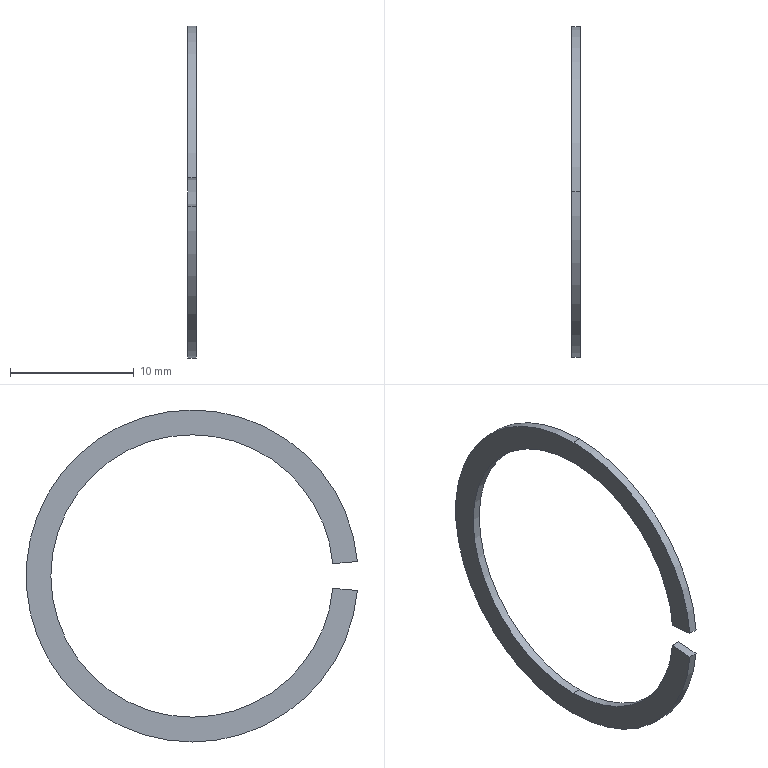Part | STEP file | 0243_Z_B6901ZZNR_2 | 1 solid | 10 faces | box 0.7 x 26.749 x 26.8 mm | volume 106.046 mm3 | cylinder 6 | plane 4 | commonest cylinder face diameters 22.8 x3 26.8 x3
STEP:
#1=CARTESIAN_POINT('',(0.,0.,0.));
#2=DIRECTION('',(0.,0.,1.));
#3=DIRECTION('',(1.,0.,0.));
#4=AXIS2_PLACEMENT_3D('',#1,#2,#3);
#5=CARTESIAN_POINT('',(1.75,0.,13.4));
#6=VERTEX_POINT('',#5);
#7=CARTESIAN_POINT('',(1.75,0.,-13.4));
#8=VERTEX_POINT('',#7);
#9=CARTESIAN_POINT('',(1.75,0.,0.));
#10=DIRECTION('',(-1.,0.,0.));
#11=DIRECTION('',(0.,0.,1.));
#12=AXIS2_PLACEMENT_3D('',#9,#10,#11);
#13=CIRCLE('',#12,13.4);
#14=CARTESIAN_POINT('',(1.05,0.,0.));
#15=DIRECTION('',(-1.,0.,0.));
#16=DIRECTION('',(0.,0.,1.));
#17=AXIS2_PLACEMENT_3D('',#14,#15,#16);
#18=CYLINDRICAL_SURFACE('',#17,13.4);
#19=CARTESIAN_POINT('',(0.,-0.7));
#20=DIRECTION('',(1.,0.));
#21=VECTOR('',#20,1.);
#22=LINE('',#19,#21);
#23=(GEOMETRIC_REPRESENTATION_CONTEXT(2)PARAMETRIC_REPRESENTATION_CONTEXT()REPRESENTATION_CONTEXT('',''));
#24=DEFINITIONAL_REPRESENTATION('',(#22),#23);
#25=PCURVE('',#18,#24);
#26=CARTESIAN_POINT('',(1.75,0.,0.));
#27=DIRECTION('',(1.,0.,0.));
#28=DIRECTION('',(0.,0.,-1.));
#29=AXIS2_PLACEMENT_3D('',#26,#27,#28);
#30=PLANE('',#29);
#31=CARTESIAN_POINT('',(-13.4,0.));
#32=CARTESIAN_POINT('',(-13.4,23.209));
#33=CARTESIAN_POINT('',(6.7,11.605));
#34=CARTESIAN_POINT('',(26.8,0.));
#35=CARTESIAN_POINT('',(6.7,-11.605));
#36=CARTESIAN_POINT('',(-13.4,-23.209));
#37=CARTESIAN_POINT('',(-13.4,0.));
#38=(BOUNDED_CURVE()B_SPLINE_CURVE(2,(#31,#32,#33,#34,#35,#36,#37),.UNSPECIFIED.,.T.,.F.)B_SPLINE_CURVE_WITH_KNOTS((1,2,2,2,2,1),(-2.094,0.,2.094,4.189,6.283,8.378),.UNSPECIFIED.)CURVE()GEOMETRIC_REPRESENTATION_ITEM()RATIONAL_B_SPLINE_CURVE((1.,0.5,1.,0.5,1.,0.5,1.))REPRESENTATION_ITEM(''));
#39=(GEOMETRIC_REPRESENTATION_CONTEXT(2)PARAMETRIC_REPRESENTATION_CONTEXT()REPRESENTATION_CONTEXT('',''));
#40=DEFINITIONAL_REPRESENTATION('',(#38),#39);
#41=PCURVE('',#30,#40);
#42=SURFACE_CURVE('',#13,(#25,#41),.PCURVE_S1.);
#43=EDGE_CURVE('',#6,#8,#42,.T.);
#44=ORIENTED_EDGE('',*,*,#43,.T.);
#45=CARTESIAN_POINT('',(1.05,0.,-13.4));
#46=VERTEX_POINT('',#45);
#47=CARTESIAN_POINT('',(1.05,0.,-13.4));
#48=DIRECTION('',(-1.,0.,0.));
#49=VECTOR('',#48,1.);
#50=LINE('',#47,#49);
#51=CARTESIAN_POINT('',(3.142,0.));
#52=DIRECTION('',(0.,1.));
#53=VECTOR('',#52,1.);
#54=LINE('',#51,#53);
#55=(GEOMETRIC_REPRESENTATION_CONTEXT(2)PARAMETRIC_REPRESENTATION_CONTEXT()REPRESENTATION_CONTEXT('',''));
#56=DEFINITIONAL_REPRESENTATION('',(#54),#55);
#57=PCURVE('',#18,#56);
#58=CARTESIAN_POINT('',(1.05,0.,0.));
#59=DIRECTION('',(-1.,0.,0.));
#60=DIRECTION('',(0.,0.,1.));
#61=AXIS2_PLACEMENT_3D('',#58,#59,#60);
#62=CYLINDRICAL_SURFACE('',#61,13.4);
#63=CARTESIAN_POINT('',(3.142,0.));
#64=DIRECTION('',(0.,1.));
#65=VECTOR('',#64,1.);
#66=LINE('',#63,#65);
#67=(GEOMETRIC_REPRESENTATION_CONTEXT(2)PARAMETRIC_REPRESENTATION_CONTEXT()REPRESENTATION_CONTEXT('',''));
#68=DEFINITIONAL_REPRESENTATION('',(#66),#67);
#69=PCURVE('',#62,#68);
#70=SURFACE_CURVE('',#50,(#57,#69),.PCURVE_S1.);
#71=EDGE_CURVE('',#8,#46,#70,.T.);
#72=ORIENTED_EDGE('',*,*,#71,.T.);
#73=CARTESIAN_POINT('',(1.05,0.,13.4));
#74=VERTEX_POINT('',#73);
#75=CARTESIAN_POINT('',(1.05,0.,0.));
#76=DIRECTION('',(1.,0.,0.));
#77=DIRECTION('',(0.,0.,1.));
#78=AXIS2_PLACEMENT_3D('',#75,#76,#77);
#79=CIRCLE('',#78,13.4);
#80=CARTESIAN_POINT('',(6.283,0.));
#81=DIRECTION('',(-1.,0.));
#82=VECTOR('',#81,1.);
#83=LINE('',#80,#82);
#84=(GEOMETRIC_REPRESENTATION_CONTEXT(2)PARAMETRIC_REPRESENTATION_CONTEXT()REPRESENTATION_CONTEXT('',''));
#85=DEFINITIONAL_REPRESENTATION('',(#83),#84);
#86=PCURVE('',#18,#85);
#87=CARTESIAN_POINT('',(1.05,0.,0.));
#88=DIRECTION('',(1.,0.,0.));
#89=DIRECTION('',(0.,0.,-1.));
#90=AXIS2_PLACEMENT_3D('',#87,#88,#89);
#91=PLANE('',#90);
#92=CARTESIAN_POINT('',(0.,0.));
#93=DIRECTION('',(-1.,0.));
#94=AXIS2_PLACEMENT_2D('',#92,#93);
#95=CIRCLE('',#94,13.4);
#96=(GEOMETRIC_REPRESENTATION_CONTEXT(2)PARAMETRIC_REPRESENTATION_CONTEXT()REPRESENTATION_CONTEXT('',''));
#97=DEFINITIONAL_REPRESENTATION('',(#95),#96);
#98=PCURVE('',#91,#97);
#99=SURFACE_CURVE('',#79,(#86,#98),.PCURVE_S1.);
#100=EDGE_CURVE('',#46,#74,#99,.T.);
#101=ORIENTED_EDGE('',*,*,#100,.T.);
#102=CARTESIAN_POINT('',(1.05,0.,13.4));
#103=DIRECTION('',(-1.,0.,0.));
#104=VECTOR('',#103,1.);
#105=LINE('',#102,#104);
#106=CARTESIAN_POINT('',(0.,0.));
#107=DIRECTION('',(0.,1.));
#108=VECTOR('',#107,1.);
#109=LINE('',#106,#108);
#110=(GEOMETRIC_REPRESENTATION_CONTEXT(2)PARAMETRIC_REPRESENTATION_CONTEXT()REPRESENTATION_CONTEXT('',''));
#111=DEFINITIONAL_REPRESENTATION('',(#109),#110);
#112=PCURVE('',#18,#111);
#113=CARTESIAN_POINT('',(1.05,0.,0.));
#114=DIRECTION('',(-1.,0.,0.));
#115=DIRECTION('',(0.,0.,1.));
#116=AXIS2_PLACEMENT_3D('',#113,#114,#115);
#117=CYLINDRICAL_SURFACE('',#116,13.4);
#118=CARTESIAN_POINT('',(6.283,0.));
#119=DIRECTION('',(0.,1.));
#120=VECTOR('',#119,1.);
#121=LINE('',#118,#120);
#122=(GEOMETRIC_REPRESENTATION_CONTEXT(2)PARAMETRIC_REPRESENTATION_CONTEXT()REPRESENTATION_CONTEXT('',''));
#123=DEFINITIONAL_REPRESENTATION('',(#121),#122);
#124=PCURVE('',#117,#123);
#125=SURFACE_CURVE('',#105,(#112,#124),.PCURVE_S1.);
#126=EDGE_CURVE('',#6,#74,#125,.T.);
#127=ORIENTED_EDGE('',*,*,#126,.F.);
#128=EDGE_LOOP('',(#44,#72,#101,#127));
#129=FACE_BOUND('',#128,.T.);
#130=ADVANCED_FACE('',(#129),#18,.T.);
#131=CARTESIAN_POINT('',(1.75,-13.349,1.168));
#132=VERTEX_POINT('',#131);
#133=CARTESIAN_POINT('',(1.75,0.,0.));
#134=DIRECTION('',(-1.,0.,0.));
#135=DIRECTION('',(0.,0.,1.));
#136=AXIS2_PLACEMENT_3D('',#133,#134,#135);
#137=CIRCLE('',#136,13.4);
#138=CARTESIAN_POINT('',(0.,-0.7));
#139=DIRECTION('',(1.,0.));
#140=VECTOR('',#139,1.);
#141=LINE('',#138,#140);
#142=(GEOMETRIC_REPRESENTATION_CONTEXT(2)PARAMETRIC_REPRESENTATION_CONTEXT()REPRESENTATION_CONTEXT('',''));
#143=DEFINITIONAL_REPRESENTATION('',(#141),#142);
#144=PCURVE('',#117,#143);
#145=CARTESIAN_POINT('',(-13.4,0.));
#146=CARTESIAN_POINT('',(-13.4,23.209));
#147=CARTESIAN_POINT('',(6.7,11.605));
#148=CARTESIAN_POINT('',(26.8,0.));
#149=CARTESIAN_POINT('',(6.7,-11.605));
#150=CARTESIAN_POINT('',(-13.4,-23.209));
#151=CARTESIAN_POINT('',(-13.4,0.));
#152=(BOUNDED_CURVE()B_SPLINE_CURVE(2,(#145,#146,#147,#148,#149,#150,#151),.UNSPECIFIED.,.T.,.F.)B_SPLINE_CURVE_WITH_KNOTS((1,2,2,2,2,1),(-2.094,0.,2.094,4.189,6.283,8.378),.UNSPECIFIED.)CURVE()GEOMETRIC_REPRESENTATION_ITEM()RATIONAL_B_SPLINE_CURVE((1.,0.5,1.,0.5,1.,0.5,1.))REPRESENTATION_ITEM(''));
#153=(GEOMETRIC_REPRESENTATION_CONTEXT(2)PARAMETRIC_REPRESENTATION_CONTEXT()REPRESENTATION_CONTEXT('',''));
#154=DEFINITIONAL_REPRESENTATION('',(#152),#153);
#155=PCURVE('',#30,#154);
#156=SURFACE_CURVE('',#137,(#144,#155),.PCURVE_S1.);
#157=EDGE_CURVE('',#132,#6,#156,.T.);
#158=ORIENTED_EDGE('',*,*,#157,.T.);
#159=ORIENTED_EDGE('',*,*,#126,.T.);
#160=CARTESIAN_POINT('',(1.05,-13.349,1.168));
#161=VERTEX_POINT('',#160);
#162=CARTESIAN_POINT('',(1.05,0.,0.));
#163=DIRECTION('',(1.,0.,0.));
#164=DIRECTION('',(0.,0.,1.));
#165=AXIS2_PLACEMENT_3D('',#162,#163,#164);
#166=CIRCLE('',#165,13.4);
#167=CARTESIAN_POINT('',(6.283,0.));
#168=DIRECTION('',(-1.,0.));
#169=VECTOR('',#168,1.);
#170=LINE('',#167,#169);
#171=(GEOMETRIC_REPRESENTATION_CONTEXT(2)PARAMETRIC_REPRESENTATION_CONTEXT()REPRESENTATION_CONTEXT('',''));
#172=DEFINITIONAL_REPRESENTATION('',(#170),#171);
#173=PCURVE('',#117,#172);
#174=CARTESIAN_POINT('',(0.,0.));
#175=DIRECTION('',(-1.,0.));
#176=AXIS2_PLACEMENT_2D('',#174,#175);
#177=CIRCLE('',#176,13.4);
#178=(GEOMETRIC_REPRESENTATION_CONTEXT(2)PARAMETRIC_REPRESENTATION_CONTEXT()REPRESENTATION_CONTEXT('',''));
#179=DEFINITIONAL_REPRESENTATION('',(#177),#178);
#180=PCURVE('',#91,#179);
#181=SURFACE_CURVE('',#166,(#173,#180),.PCURVE_S1.);
#182=EDGE_CURVE('',#74,#161,#181,.T.);
#183=ORIENTED_EDGE('',*,*,#182,.T.);
#184=CARTESIAN_POINT('',(1.05,-13.349,1.168));
#185=DIRECTION('',(-1.,0.,0.));
#186=VECTOR('',#185,1.);
#187=LINE('',#184,#186);
#188=CARTESIAN_POINT('',(4.8,0.));
#189=DIRECTION('',(0.,1.));
#190=VECTOR('',#189,1.);
#191=LINE('',#188,#190);
#192=(GEOMETRIC_REPRESENTATION_CONTEXT(2)PARAMETRIC_REPRESENTATION_CONTEXT()REPRESENTATION_CONTEXT('',''));
#193=DEFINITIONAL_REPRESENTATION('',(#191),#192);
#194=PCURVE('',#117,#193);
#195=CARTESIAN_POINT('',(1.05,-11.357,0.9936));
#196=DIRECTION('',(0.,-0.08716,-0.9962));
#197=DIRECTION('',(0.,0.9962,-0.08716));
#198=AXIS2_PLACEMENT_3D('',#195,#196,#197);
#199=PLANE('',#198);
#200=CARTESIAN_POINT('',(-2.,0.));
#201=DIRECTION('',(0.,-1.));
#202=VECTOR('',#201,1.);
#203=LINE('',#200,#202);
#204=(GEOMETRIC_REPRESENTATION_CONTEXT(2)PARAMETRIC_REPRESENTATION_CONTEXT()REPRESENTATION_CONTEXT('',''));
#205=DEFINITIONAL_REPRESENTATION('',(#203),#204);
#206=PCURVE('',#199,#205);
#207=SURFACE_CURVE('',#187,(#194,#206),.PCURVE_S1.);
#208=EDGE_CURVE('',#132,#161,#207,.T.);
#209=ORIENTED_EDGE('',*,*,#208,.F.);
#210=EDGE_LOOP('',(#158,#159,#183,#209));
#211=FACE_BOUND('',#210,.T.);
#212=ADVANCED_FACE('',(#211),#117,.T.);
#213=CARTESIAN_POINT('',(1.75,-11.357,-0.9936));
#214=VERTEX_POINT('',#213);
#215=CARTESIAN_POINT('',(1.05,-11.357,-0.9936));
#216=VERTEX_POINT('',#215);
#217=CARTESIAN_POINT('',(1.05,-11.357,-0.9936));
#218=DIRECTION('',(-1.,0.,0.));
#219=VECTOR('',#218,1.);
#220=LINE('',#217,#219);
#221=CARTESIAN_POINT('',(1.05,0.,0.));
#222=DIRECTION('',(-1.,0.,0.));
#223=DIRECTION('',(0.,0.,1.));
#224=AXIS2_PLACEMENT_3D('',#221,#222,#223);
#225=CYLINDRICAL_SURFACE('',#224,11.4);
#226=CARTESIAN_POINT('',(4.625,0.));
#227=DIRECTION('',(0.,1.));
#228=VECTOR('',#227,1.);
#229=LINE('',#226,#228);
#230=(GEOMETRIC_REPRESENTATION_CONTEXT(2)PARAMETRIC_REPRESENTATION_CONTEXT()REPRESENTATION_CONTEXT('',''));
#231=DEFINITIONAL_REPRESENTATION('',(#229),#230);
#232=PCURVE('',#225,#231);
#233=CARTESIAN_POINT('',(1.05,-13.349,-1.168));
#234=DIRECTION('',(0.,-0.08716,0.9962));
#235=DIRECTION('',(0.,-0.9962,-0.08716));
#236=AXIS2_PLACEMENT_3D('',#233,#234,#235);
#237=PLANE('',#236);
#238=CARTESIAN_POINT('',(-2.,0.));
#239=DIRECTION('',(0.,-1.));
#240=VECTOR('',#239,1.);
#241=LINE('',#238,#240);
#242=(GEOMETRIC_REPRESENTATION_CONTEXT(2)PARAMETRIC_REPRESENTATION_CONTEXT()REPRESENTATION_CONTEXT('',''));
#243=DEFINITIONAL_REPRESENTATION('',(#241),#242);
#244=PCURVE('',#237,#243);
#245=SURFACE_CURVE('',#220,(#232,#244),.PCURVE_S1.);
#246=EDGE_CURVE('',#214,#216,#245,.T.);
#247=ORIENTED_EDGE('',*,*,#246,.T.);
#248=CARTESIAN_POINT('',(1.05,0.,-11.4));
#249=VERTEX_POINT('',#248);
#250=CARTESIAN_POINT('',(1.05,0.,0.));
#251=DIRECTION('',(-1.,0.,0.));
#252=DIRECTION('',(0.,0.,1.));
#253=AXIS2_PLACEMENT_3D('',#250,#251,#252);
#254=CIRCLE('',#253,11.4);
#255=CARTESIAN_POINT('',(0.,0.));
#256=DIRECTION('',(1.,0.));
#257=VECTOR('',#256,1.);
#258=LINE('',#255,#257);
#259=(GEOMETRIC_REPRESENTATION_CONTEXT(2)PARAMETRIC_REPRESENTATION_CONTEXT()REPRESENTATION_CONTEXT('',''));
#260=DEFINITIONAL_REPRESENTATION('',(#258),#259);
#261=PCURVE('',#225,#260);
#262=CARTESIAN_POINT('',(-11.4,0.));
#263=CARTESIAN_POINT('',(-11.4,19.745));
#264=CARTESIAN_POINT('',(5.7,9.873));
#265=CARTESIAN_POINT('',(22.8,0.));
#266=CARTESIAN_POINT('',(5.7,-9.873));
#267=CARTESIAN_POINT('',(-11.4,-19.745));
#268=CARTESIAN_POINT('',(-11.4,0.));
#269=(BOUNDED_CURVE()B_SPLINE_CURVE(2,(#262,#263,#264,#265,#266,#267,#268),.UNSPECIFIED.,.T.,.F.)B_SPLINE_CURVE_WITH_KNOTS((1,2,2,2,2,1),(-2.094,0.,2.094,4.189,6.283,8.378),.UNSPECIFIED.)CURVE()GEOMETRIC_REPRESENTATION_ITEM()RATIONAL_B_SPLINE_CURVE((1.,0.5,1.,0.5,1.,0.5,1.))REPRESENTATION_ITEM(''));
#270=(GEOMETRIC_REPRESENTATION_CONTEXT(2)PARAMETRIC_REPRESENTATION_CONTEXT()REPRESENTATION_CONTEXT('',''));
#271=DEFINITIONAL_REPRESENTATION('',(#269),#270);
#272=PCURVE('',#91,#271);
#273=SURFACE_CURVE('',#254,(#261,#272),.PCURVE_S1.);
#274=EDGE_CURVE('',#249,#216,#273,.T.);
#275=ORIENTED_EDGE('',*,*,#274,.F.);
#276=CARTESIAN_POINT('',(1.75,0.,-11.4));
#277=VERTEX_POINT('',#276);
#278=CARTESIAN_POINT('',(1.05,0.,-11.4));
#279=DIRECTION('',(-1.,0.,0.));
#280=VECTOR('',#279,1.);
#281=LINE('',#278,#280);
#282=CARTESIAN_POINT('',(3.142,0.));
#283=DIRECTION('',(0.,1.));
#284=VECTOR('',#283,1.);
#285=LINE('',#282,#284);
#286=(GEOMETRIC_REPRESENTATION_CONTEXT(2)PARAMETRIC_REPRESENTATION_CONTEXT()REPRESENTATION_CONTEXT('',''));
#287=DEFINITIONAL_REPRESENTATION('',(#285),#286);
#288=PCURVE('',#225,#287);
#289=CARTESIAN_POINT('',(1.05,0.,0.));
#290=DIRECTION('',(-1.,0.,0.));
#291=DIRECTION('',(0.,0.,1.));
#292=AXIS2_PLACEMENT_3D('',#289,#290,#291);
#293=CYLINDRICAL_SURFACE('',#292,11.4);
#294=CARTESIAN_POINT('',(3.142,0.));
#295=DIRECTION('',(0.,1.));
#296=VECTOR('',#295,1.);
#297=LINE('',#294,#296);
#298=(GEOMETRIC_REPRESENTATION_CONTEXT(2)PARAMETRIC_REPRESENTATION_CONTEXT()REPRESENTATION_CONTEXT('',''));
#299=DEFINITIONAL_REPRESENTATION('',(#297),#298);
#300=PCURVE('',#293,#299);
#301=SURFACE_CURVE('',#281,(#288,#300),.PCURVE_S1.);
#302=EDGE_CURVE('',#277,#249,#301,.T.);
#303=ORIENTED_EDGE('',*,*,#302,.F.);
#304=CARTESIAN_POINT('',(1.75,0.,0.));
#305=DIRECTION('',(-1.,0.,0.));
#306=DIRECTION('',(0.,0.,1.));
#307=AXIS2_PLACEMENT_3D('',#304,#305,#306);
#308=CIRCLE('',#307,11.4);
#309=CARTESIAN_POINT('',(0.,-0.7));
#310=DIRECTION('',(1.,0.));
#311=VECTOR('',#310,1.);
#312=LINE('',#309,#311);
#313=(GEOMETRIC_REPRESENTATION_CONTEXT(2)PARAMETRIC_REPRESENTATION_CONTEXT()REPRESENTATION_CONTEXT('',''));
#314=DEFINITIONAL_REPRESENTATION('',(#312),#313);
#315=PCURVE('',#225,#314);
#316=CARTESIAN_POINT('',(-11.4,0.));
#317=CARTESIAN_POINT('',(-11.4,19.745));
#318=CARTESIAN_POINT('',(5.7,9.873));
#319=CARTESIAN_POINT('',(22.8,0.));
#320=CARTESIAN_POINT('',(5.7,-9.873));
#321=CARTESIAN_POINT('',(-11.4,-19.745));
#322=CARTESIAN_POINT('',(-11.4,0.));
#323=(BOUNDED_CURVE()B_SPLINE_CURVE(2,(#316,#317,#318,#319,#320,#321,#322),.UNSPECIFIED.,.T.,.F.)B_SPLINE_CURVE_WITH_KNOTS((1,2,2,2,2,1),(-2.094,0.,2.094,4.189,6.283,8.378),.UNSPECIFIED.)CURVE()GEOMETRIC_REPRESENTATION_ITEM()RATIONAL_B_SPLINE_CURVE((1.,0.5,1.,0.5,1.,0.5,1.))REPRESENTATION_ITEM(''));
#324=(GEOMETRIC_REPRESENTATION_CONTEXT(2)PARAMETRIC_REPRESENTATION_CONTEXT()REPRESENTATION_CONTEXT('',''));
#325=DEFINITIONAL_REPRESENTATION('',(#323),#324);
#326=PCURVE('',#30,#325);
#327=SURFACE_CURVE('',#308,(#315,#326),.PCURVE_S1.);
#328=EDGE_CURVE('',#277,#214,#327,.T.);
#329=ORIENTED_EDGE('',*,*,#328,.T.);
#330=EDGE_LOOP('',(#247,#275,#303,#329));
#331=FACE_BOUND('',#330,.F.);
#332=ADVANCED_FACE('',(#331),#225,.F.);
#333=CARTESIAN_POINT('',(1.05,0.,11.4));
#334=VERTEX_POINT('',#333);
#335=CARTESIAN_POINT('',(1.05,0.,0.));
#336=DIRECTION('',(-1.,0.,0.));
#337=DIRECTION('',(0.,0.,1.));
#338=AXIS2_PLACEMENT_3D('',#335,#336,#337);
#339=CIRCLE('',#338,11.4);
#340=CARTESIAN_POINT('',(0.,0.));
#341=DIRECTION('',(1.,0.));
#342=VECTOR('',#341,1.);
#343=LINE('',#340,#342);
#344=(GEOMETRIC_REPRESENTATION_CONTEXT(2)PARAMETRIC_REPRESENTATION_CONTEXT()REPRESENTATION_CONTEXT('',''));
#345=DEFINITIONAL_REPRESENTATION('',(#343),#344);
#346=PCURVE('',#293,#345);
#347=CARTESIAN_POINT('',(-11.4,0.));
#348=CARTESIAN_POINT('',(-11.4,19.745));
#349=CARTESIAN_POINT('',(5.7,9.873));
#350=CARTESIAN_POINT('',(22.8,0.));
#351=CARTESIAN_POINT('',(5.7,-9.873));
#352=CARTESIAN_POINT('',(-11.4,-19.745));
#353=CARTESIAN_POINT('',(-11.4,0.));
#354=(BOUNDED_CURVE()B_SPLINE_CURVE(2,(#347,#348,#349,#350,#351,#352,#353),.UNSPECIFIED.,.T.,.F.)B_SPLINE_CURVE_WITH_KNOTS((1,2,2,2,2,1),(-2.094,0.,2.094,4.189,6.283,8.378),.UNSPECIFIED.)CURVE()GEOMETRIC_REPRESENTATION_ITEM()RATIONAL_B_SPLINE_CURVE((1.,0.5,1.,0.5,1.,0.5,1.))REPRESENTATION_ITEM(''));
#355=(GEOMETRIC_REPRESENTATION_CONTEXT(2)PARAMETRIC_REPRESENTATION_CONTEXT()REPRESENTATION_CONTEXT('',''));
#356=DEFINITIONAL_REPRESENTATION('',(#354),#355);
#357=PCURVE('',#91,#356);
#358=SURFACE_CURVE('',#339,(#346,#357),.PCURVE_S1.);
#359=EDGE_CURVE('',#334,#249,#358,.T.);
#360=ORIENTED_EDGE('',*,*,#359,.F.);
#361=CARTESIAN_POINT('',(1.75,0.,11.4));
#362=VERTEX_POINT('',#361);
#363=CARTESIAN_POINT('',(1.05,0.,11.4));
#364=DIRECTION('',(-1.,0.,0.));
#365=VECTOR('',#364,1.);
#366=LINE('',#363,#365);
#367=CARTESIAN_POINT('',(0.,0.));
#368=DIRECTION('',(0.,1.));
#369=VECTOR('',#368,1.);
#370=LINE('',#367,#369);
#371=(GEOMETRIC_REPRESENTATION_CONTEXT(2)PARAMETRIC_REPRESENTATION_CONTEXT()REPRESENTATION_CONTEXT('',''));
#372=DEFINITIONAL_REPRESENTATION('',(#370),#371);
#373=PCURVE('',#293,#372);
#374=CARTESIAN_POINT('',(1.05,0.,0.));
#375=DIRECTION('',(-1.,0.,0.));
#376=DIRECTION('',(0.,0.,1.));
#377=AXIS2_PLACEMENT_3D('',#374,#375,#376);
#378=CYLINDRICAL_SURFACE('',#377,11.4);
#379=CARTESIAN_POINT('',(6.283,0.));
#380=DIRECTION('',(0.,1.));
#381=VECTOR('',#380,1.);
#382=LINE('',#379,#381);
#383=(GEOMETRIC_REPRESENTATION_CONTEXT(2)PARAMETRIC_REPRESENTATION_CONTEXT()REPRESENTATION_CONTEXT('',''));
#384=DEFINITIONAL_REPRESENTATION('',(#382),#383);
#385=PCURVE('',#378,#384);
#386=SURFACE_CURVE('',#366,(#373,#385),.PCURVE_S1.);
#387=EDGE_CURVE('',#362,#334,#386,.T.);
#388=ORIENTED_EDGE('',*,*,#387,.F.);
#389=CARTESIAN_POINT('',(1.75,0.,0.));
#390=DIRECTION('',(-1.,0.,0.));
#391=DIRECTION('',(0.,0.,1.));
#392=AXIS2_PLACEMENT_3D('',#389,#390,#391);
#393=CIRCLE('',#392,11.4);
#394=CARTESIAN_POINT('',(0.,-0.7));
#395=DIRECTION('',(1.,0.));
#396=VECTOR('',#395,1.);
#397=LINE('',#394,#396);
#398=(GEOMETRIC_REPRESENTATION_CONTEXT(2)PARAMETRIC_REPRESENTATION_CONTEXT()REPRESENTATION_CONTEXT('',''));
#399=DEFINITIONAL_REPRESENTATION('',(#397),#398);
#400=PCURVE('',#293,#399);
#401=CARTESIAN_POINT('',(-11.4,0.));
#402=CARTESIAN_POINT('',(-11.4,19.745));
#403=CARTESIAN_POINT('',(5.7,9.873));
#404=CARTESIAN_POINT('',(22.8,0.));
#405=CARTESIAN_POINT('',(5.7,-9.873));
#406=CARTESIAN_POINT('',(-11.4,-19.745));
#407=CARTESIAN_POINT('',(-11.4,0.));
#408=(BOUNDED_CURVE()B_SPLINE_CURVE(2,(#401,#402,#403,#404,#405,#406,#407),.UNSPECIFIED.,.T.,.F.)B_SPLINE_CURVE_WITH_KNOTS((1,2,2,2,2,1),(-2.094,0.,2.094,4.189,6.283,8.378),.UNSPECIFIED.)CURVE()GEOMETRIC_REPRESENTATION_ITEM()RATIONAL_B_SPLINE_CURVE((1.,0.5,1.,0.5,1.,0.5,1.))REPRESENTATION_ITEM(''));
#409=(GEOMETRIC_REPRESENTATION_CONTEXT(2)PARAMETRIC_REPRESENTATION_CONTEXT()REPRESENTATION_CONTEXT('',''));
#410=DEFINITIONAL_REPRESENTATION('',(#408),#409);
#411=PCURVE('',#30,#410);
#412=SURFACE_CURVE('',#393,(#400,#411),.PCURVE_S1.);
#413=EDGE_CURVE('',#362,#277,#412,.T.);
#414=ORIENTED_EDGE('',*,*,#413,.T.);
#415=ORIENTED_EDGE('',*,*,#302,.T.);
#416=EDGE_LOOP('',(#360,#388,#414,#415));
#417=FACE_BOUND('',#416,.F.);
#418=ADVANCED_FACE('',(#417),#293,.F.);
#419=CARTESIAN_POINT('',(1.05,-13.349,-1.168));
#420=VERTEX_POINT('',#419);
#421=CARTESIAN_POINT('',(1.05,-11.357,-0.9936));
#422=DIRECTION('',(0.,-0.9962,-0.08716));
#423=VECTOR('',#422,1.);
#424=LINE('',#421,#423);
#425=CARTESIAN_POINT('',(0.9936,-11.357));
#426=DIRECTION('',(0.08716,-0.9962));
#427=VECTOR('',#426,1.);
#428=LINE('',#425,#427);
#429=(GEOMETRIC_REPRESENTATION_CONTEXT(2)PARAMETRIC_REPRESENTATION_CONTEXT()REPRESENTATION_CONTEXT('',''));
#430=DEFINITIONAL_REPRESENTATION('',(#428),#429);
#431=PCURVE('',#91,#430);
#432=CARTESIAN_POINT('',(-2.,0.));
#433=DIRECTION('',(1.,0.));
#434=VECTOR('',#433,1.);
#435=LINE('',#432,#434);
#436=(GEOMETRIC_REPRESENTATION_CONTEXT(2)PARAMETRIC_REPRESENTATION_CONTEXT()REPRESENTATION_CONTEXT('',''));
#437=DEFINITIONAL_REPRESENTATION('',(#435),#436);
#438=PCURVE('',#237,#437);
#439=SURFACE_CURVE('',#424,(#431,#438),.PCURVE_S1.);
#440=EDGE_CURVE('',#216,#420,#439,.T.);
#441=ORIENTED_EDGE('',*,*,#440,.F.);
#442=ORIENTED_EDGE('',*,*,#274,.F.);
#443=ORIENTED_EDGE('',*,*,#359,.F.);
#444=CARTESIAN_POINT('',(1.05,-11.357,0.9936));
#445=VERTEX_POINT('',#444);
#446=CARTESIAN_POINT('',(1.05,0.,0.));
#447=DIRECTION('',(-1.,0.,0.));
#448=DIRECTION('',(0.,0.,1.));
#449=AXIS2_PLACEMENT_3D('',#446,#447,#448);
#450=CIRCLE('',#449,11.4);
#451=CARTESIAN_POINT('',(-11.4,0.));
#452=CARTESIAN_POINT('',(-11.4,19.745));
#453=CARTESIAN_POINT('',(5.7,9.873));
#454=CARTESIAN_POINT('',(22.8,0.));
#455=CARTESIAN_POINT('',(5.7,-9.873));
#456=CARTESIAN_POINT('',(-11.4,-19.745));
#457=CARTESIAN_POINT('',(-11.4,0.));
#458=(BOUNDED_CURVE()B_SPLINE_CURVE(2,(#451,#452,#453,#454,#455,#456,#457),.UNSPECIFIED.,.T.,.F.)B_SPLINE_CURVE_WITH_KNOTS((1,2,2,2,2,1),(-2.094,0.,2.094,4.189,6.283,8.378),.UNSPECIFIED.)CURVE()GEOMETRIC_REPRESENTATION_ITEM()RATIONAL_B_SPLINE_CURVE((1.,0.5,1.,0.5,1.,0.5,1.))REPRESENTATION_ITEM(''));
#459=(GEOMETRIC_REPRESENTATION_CONTEXT(2)PARAMETRIC_REPRESENTATION_CONTEXT()REPRESENTATION_CONTEXT('',''));
#460=DEFINITIONAL_REPRESENTATION('',(#458),#459);
#461=PCURVE('',#91,#460);
#462=CARTESIAN_POINT('',(0.,0.));
#463=DIRECTION('',(1.,0.));
#464=VECTOR('',#463,1.);
#465=LINE('',#462,#464);
#466=(GEOMETRIC_REPRESENTATION_CONTEXT(2)PARAMETRIC_REPRESENTATION_CONTEXT()REPRESENTATION_CONTEXT('',''));
#467=DEFINITIONAL_REPRESENTATION('',(#465),#466);
#468=PCURVE('',#378,#467);
#469=SURFACE_CURVE('',#450,(#461,#468),.PCURVE_S1.);
#470=EDGE_CURVE('',#445,#334,#469,.T.);
#471=ORIENTED_EDGE('',*,*,#470,.F.);
#472=CARTESIAN_POINT('',(1.05,-13.349,1.168));
#473=DIRECTION('',(0.,0.9962,-0.08716));
#474=VECTOR('',#473,1.);
#475=LINE('',#472,#474);
#476=CARTESIAN_POINT('',(-1.168,-13.349));
#477=DIRECTION('',(0.08716,0.9962));
#478=VECTOR('',#477,1.);
#479=LINE('',#476,#478);
#480=(GEOMETRIC_REPRESENTATION_CONTEXT(2)PARAMETRIC_REPRESENTATION_CONTEXT()REPRESENTATION_CONTEXT('',''));
#481=DEFINITIONAL_REPRESENTATION('',(#479),#480);
#482=PCURVE('',#91,#481);
#483=CARTESIAN_POINT('',(-2.,0.));
#484=DIRECTION('',(1.,0.));
#485=VECTOR('',#484,1.);
#486=LINE('',#483,#485);
#487=(GEOMETRIC_REPRESENTATION_CONTEXT(2)PARAMETRIC_REPRESENTATION_CONTEXT()REPRESENTATION_CONTEXT('',''));
#488=DEFINITIONAL_REPRESENTATION('',(#486),#487);
#489=PCURVE('',#199,#488);
#490=SURFACE_CURVE('',#475,(#482,#489),.PCURVE_S1.);
#491=EDGE_CURVE('',#161,#445,#490,.T.);
#492=ORIENTED_EDGE('',*,*,#491,.F.);
#493=ORIENTED_EDGE('',*,*,#182,.F.);
#494=ORIENTED_EDGE('',*,*,#100,.F.);
#495=CARTESIAN_POINT('',(1.05,0.,0.));
#496=DIRECTION('',(1.,0.,0.));
#497=DIRECTION('',(0.,0.,1.));
#498=AXIS2_PLACEMENT_3D('',#495,#496,#497);
#499=CIRCLE('',#498,13.4);
#500=CARTESIAN_POINT('',(0.,0.));
#501=DIRECTION('',(-1.,0.));
#502=AXIS2_PLACEMENT_2D('',#500,#501);
#503=CIRCLE('',#502,13.4);
#504=(GEOMETRIC_REPRESENTATION_CONTEXT(2)PARAMETRIC_REPRESENTATION_CONTEXT()REPRESENTATION_CONTEXT('',''));
#505=DEFINITIONAL_REPRESENTATION('',(#503),#504);
#506=PCURVE('',#91,#505);
#507=CARTESIAN_POINT('',(6.283,0.));
#508=DIRECTION('',(-1.,0.));
#509=VECTOR('',#508,1.);
#510=LINE('',#507,#509);
#511=(GEOMETRIC_REPRESENTATION_CONTEXT(2)PARAMETRIC_REPRESENTATION_CONTEXT()REPRESENTATION_CONTEXT('',''));
#512=DEFINITIONAL_REPRESENTATION('',(#510),#511);
#513=PCURVE('',#62,#512);
#514=SURFACE_CURVE('',#499,(#506,#513),.PCURVE_S1.);
#515=EDGE_CURVE('',#420,#46,#514,.T.);
#516=ORIENTED_EDGE('',*,*,#515,.F.);
#517=EDGE_LOOP('',(#441,#442,#443,#471,#492,#493,#494,#516));
#518=FACE_BOUND('',#517,.T.);
#519=ADVANCED_FACE('',(#518),#91,.F.);
#520=ORIENTED_EDGE('',*,*,#71,.F.);
#521=CARTESIAN_POINT('',(1.75,-13.349,-1.168));
#522=VERTEX_POINT('',#521);
#523=CARTESIAN_POINT('',(1.75,0.,0.));
#524=DIRECTION('',(-1.,0.,0.));
#525=DIRECTION('',(0.,0.,1.));
#526=AXIS2_PLACEMENT_3D('',#523,#524,#525);
#527=CIRCLE('',#526,13.4);
#528=CARTESIAN_POINT('',(0.,-0.7));
#529=DIRECTION('',(1.,0.));
#530=VECTOR('',#529,1.);
#531=LINE('',#528,#530);
#532=(GEOMETRIC_REPRESENTATION_CONTEXT(2)PARAMETRIC_REPRESENTATION_CONTEXT()REPRESENTATION_CONTEXT('',''));
#533=DEFINITIONAL_REPRESENTATION('',(#531),#532);
#534=PCURVE('',#62,#533);
#535=CARTESIAN_POINT('',(-13.4,0.));
#536=CARTESIAN_POINT('',(-13.4,23.209));
#537=CARTESIAN_POINT('',(6.7,11.605));
#538=CARTESIAN_POINT('',(26.8,0.));
#539=CARTESIAN_POINT('',(6.7,-11.605));
#540=CARTESIAN_POINT('',(-13.4,-23.209));
#541=CARTESIAN_POINT('',(-13.4,0.));
#542=(BOUNDED_CURVE()B_SPLINE_CURVE(2,(#535,#536,#537,#538,#539,#540,#541),.UNSPECIFIED.,.T.,.F.)B_SPLINE_CURVE_WITH_KNOTS((1,2,2,2,2,1),(-2.094,0.,2.094,4.189,6.283,8.378),.UNSPECIFIED.)CURVE()GEOMETRIC_REPRESENTATION_ITEM()RATIONAL_B_SPLINE_CURVE((1.,0.5,1.,0.5,1.,0.5,1.))REPRESENTATION_ITEM(''));
#543=(GEOMETRIC_REPRESENTATION_CONTEXT(2)PARAMETRIC_REPRESENTATION_CONTEXT()REPRESENTATION_CONTEXT('',''));
#544=DEFINITIONAL_REPRESENTATION('',(#542),#543);
#545=PCURVE('',#30,#544);
#546=SURFACE_CURVE('',#527,(#534,#545),.PCURVE_S1.);
#547=EDGE_CURVE('',#8,#522,#546,.T.);
#548=ORIENTED_EDGE('',*,*,#547,.T.);
#549=CARTESIAN_POINT('',(1.05,-13.349,-1.168));
#550=DIRECTION('',(-1.,0.,0.));
#551=VECTOR('',#550,1.);
#552=LINE('',#549,#551);
#553=CARTESIAN_POINT('',(4.625,0.));
#554=DIRECTION('',(0.,1.));
#555=VECTOR('',#554,1.);
#556=LINE('',#553,#555);
#557=(GEOMETRIC_REPRESENTATION_CONTEXT(2)PARAMETRIC_REPRESENTATION_CONTEXT()REPRESENTATION_CONTEXT('',''));
#558=DEFINITIONAL_REPRESENTATION('',(#556),#557);
#559=PCURVE('',#62,#558);
#560=CARTESIAN_POINT('',(0.,0.));
#561=DIRECTION('',(0.,-1.));
#562=VECTOR('',#561,1.);
#563=LINE('',#560,#562);
#564=(GEOMETRIC_REPRESENTATION_CONTEXT(2)PARAMETRIC_REPRESENTATION_CONTEXT()REPRESENTATION_CONTEXT('',''));
#565=DEFINITIONAL_REPRESENTATION('',(#563),#564);
#566=PCURVE('',#237,#565);
#567=SURFACE_CURVE('',#552,(#559,#566),.PCURVE_S1.);
#568=EDGE_CURVE('',#522,#420,#567,.T.);
#569=ORIENTED_EDGE('',*,*,#568,.T.);
#570=ORIENTED_EDGE('',*,*,#515,.T.);
#571=EDGE_LOOP('',(#520,#548,#569,#570));
#572=FACE_BOUND('',#571,.T.);
#573=ADVANCED_FACE('',(#572),#62,.T.);
#574=ORIENTED_EDGE('',*,*,#440,.T.);
#575=ORIENTED_EDGE('',*,*,#568,.F.);
#576=CARTESIAN_POINT('',(1.75,-13.349,-1.168));
#577=DIRECTION('',(0.,0.9962,0.08716));
#578=VECTOR('',#577,1.);
#579=LINE('',#576,#578);
#580=CARTESIAN_POINT('',(0.,0.7));
#581=DIRECTION('',(-1.,0.));
#582=VECTOR('',#581,1.);
#583=LINE('',#580,#582);
#584=(GEOMETRIC_REPRESENTATION_CONTEXT(2)PARAMETRIC_REPRESENTATION_CONTEXT()REPRESENTATION_CONTEXT('',''));
#585=DEFINITIONAL_REPRESENTATION('',(#583),#584);
#586=PCURVE('',#237,#585);
#587=CARTESIAN_POINT('',(1.168,-13.349));
#588=DIRECTION('',(-0.08716,0.9962));
#589=VECTOR('',#588,1.);
#590=LINE('',#587,#589);
#591=(GEOMETRIC_REPRESENTATION_CONTEXT(2)PARAMETRIC_REPRESENTATION_CONTEXT()REPRESENTATION_CONTEXT('',''));
#592=DEFINITIONAL_REPRESENTATION('',(#590),#591);
#593=PCURVE('',#30,#592);
#594=SURFACE_CURVE('',#579,(#586,#593),.PCURVE_S1.);
#595=EDGE_CURVE('',#522,#214,#594,.T.);
#596=ORIENTED_EDGE('',*,*,#595,.T.);
#597=ORIENTED_EDGE('',*,*,#246,.T.);
#598=EDGE_LOOP('',(#574,#575,#596,#597));
#599=FACE_BOUND('',#598,.T.);
#600=ADVANCED_FACE('',(#599),#237,.T.);
#601=ORIENTED_EDGE('',*,*,#470,.F.);
#602=CARTESIAN_POINT('',(1.75,-11.357,0.9936));
#603=VERTEX_POINT('',#602);
#604=CARTESIAN_POINT('',(1.05,-11.357,0.9936));
#605=DIRECTION('',(1.,0.,0.));
#606=VECTOR('',#605,1.);
#607=LINE('',#604,#606);
#608=CARTESIAN_POINT('',(4.8,0.));
#609=DIRECTION('',(0.,-1.));
#610=VECTOR('',#609,1.);
#611=LINE('',#608,#610);
#612=(GEOMETRIC_REPRESENTATION_CONTEXT(2)PARAMETRIC_REPRESENTATION_CONTEXT()REPRESENTATION_CONTEXT('',''));
#613=DEFINITIONAL_REPRESENTATION('',(#611),#612);
#614=PCURVE('',#378,#613);
#615=CARTESIAN_POINT('',(0.,0.));
#616=DIRECTION('',(0.,1.));
#617=VECTOR('',#616,1.);
#618=LINE('',#615,#617);
#619=(GEOMETRIC_REPRESENTATION_CONTEXT(2)PARAMETRIC_REPRESENTATION_CONTEXT()REPRESENTATION_CONTEXT('',''));
#620=DEFINITIONAL_REPRESENTATION('',(#618),#619);
#621=PCURVE('',#199,#620);
#622=SURFACE_CURVE('',#607,(#614,#621),.PCURVE_S1.);
#623=EDGE_CURVE('',#445,#603,#622,.T.);
#624=ORIENTED_EDGE('',*,*,#623,.T.);
#625=CARTESIAN_POINT('',(1.75,0.,0.));
#626=DIRECTION('',(-1.,0.,0.));
#627=DIRECTION('',(0.,0.,1.));
#628=AXIS2_PLACEMENT_3D('',#625,#626,#627);
#629=CIRCLE('',#628,11.4);
#630=CARTESIAN_POINT('',(0.,-0.7));
#631=DIRECTION('',(1.,0.));
#632=VECTOR('',#631,1.);
#633=LINE('',#630,#632);
#634=(GEOMETRIC_REPRESENTATION_CONTEXT(2)PARAMETRIC_REPRESENTATION_CONTEXT()REPRESENTATION_CONTEXT('',''));
#635=DEFINITIONAL_REPRESENTATION('',(#633),#634);
#636=PCURVE('',#378,#635);
#637=CARTESIAN_POINT('',(-11.4,0.));
#638=CARTESIAN_POINT('',(-11.4,19.745));
#639=CARTESIAN_POINT('',(5.7,9.873));
#640=CARTESIAN_POINT('',(22.8,0.));
#641=CARTESIAN_POINT('',(5.7,-9.873));
#642=CARTESIAN_POINT('',(-11.4,-19.745));
#643=CARTESIAN_POINT('',(-11.4,0.));
#644=(BOUNDED_CURVE()B_SPLINE_CURVE(2,(#637,#638,#639,#640,#641,#642,#643),.UNSPECIFIED.,.T.,.F.)B_SPLINE_CURVE_WITH_KNOTS((1,2,2,2,2,1),(-2.094,0.,2.094,4.189,6.283,8.378),.UNSPECIFIED.)CURVE()GEOMETRIC_REPRESENTATION_ITEM()RATIONAL_B_SPLINE_CURVE((1.,0.5,1.,0.5,1.,0.5,1.))REPRESENTATION_ITEM(''));
#645=(GEOMETRIC_REPRESENTATION_CONTEXT(2)PARAMETRIC_REPRESENTATION_CONTEXT()REPRESENTATION_CONTEXT('',''));
#646=DEFINITIONAL_REPRESENTATION('',(#644),#645);
#647=PCURVE('',#30,#646);
#648=SURFACE_CURVE('',#629,(#636,#647),.PCURVE_S1.);
#649=EDGE_CURVE('',#603,#362,#648,.T.);
#650=ORIENTED_EDGE('',*,*,#649,.T.);
#651=ORIENTED_EDGE('',*,*,#387,.T.);
#652=EDGE_LOOP('',(#601,#624,#650,#651));
#653=FACE_BOUND('',#652,.F.);
#654=ADVANCED_FACE('',(#653),#378,.F.);
#655=ORIENTED_EDGE('',*,*,#491,.T.);
#656=ORIENTED_EDGE('',*,*,#623,.T.);
#657=CARTESIAN_POINT('',(1.75,-11.357,0.9936));
#658=DIRECTION('',(0.,-0.9962,0.08716));
#659=VECTOR('',#658,1.);
#660=LINE('',#657,#659);
#661=CARTESIAN_POINT('',(0.,0.7));
#662=DIRECTION('',(-1.,0.));
#663=VECTOR('',#662,1.);
#664=LINE('',#661,#663);
#665=(GEOMETRIC_REPRESENTATION_CONTEXT(2)PARAMETRIC_REPRESENTATION_CONTEXT()REPRESENTATION_CONTEXT('',''));
#666=DEFINITIONAL_REPRESENTATION('',(#664),#665);
#667=PCURVE('',#199,#666);
#668=CARTESIAN_POINT('',(-0.9936,-11.357));
#669=DIRECTION('',(-0.08716,-0.9962));
#670=VECTOR('',#669,1.);
#671=LINE('',#668,#670);
#672=(GEOMETRIC_REPRESENTATION_CONTEXT(2)PARAMETRIC_REPRESENTATION_CONTEXT()REPRESENTATION_CONTEXT('',''));
#673=DEFINITIONAL_REPRESENTATION('',(#671),#672);
#674=PCURVE('',#30,#673);
#675=SURFACE_CURVE('',#660,(#667,#674),.PCURVE_S1.);
#676=EDGE_CURVE('',#603,#132,#675,.T.);
#677=ORIENTED_EDGE('',*,*,#676,.T.);
#678=ORIENTED_EDGE('',*,*,#208,.T.);
#679=EDGE_LOOP('',(#655,#656,#677,#678));
#680=FACE_BOUND('',#679,.T.);
#681=ADVANCED_FACE('',(#680),#199,.T.);
#682=ORIENTED_EDGE('',*,*,#676,.F.);
#683=ORIENTED_EDGE('',*,*,#649,.T.);
#684=ORIENTED_EDGE('',*,*,#413,.T.);
#685=ORIENTED_EDGE('',*,*,#328,.T.);
#686=ORIENTED_EDGE('',*,*,#595,.F.);
#687=ORIENTED_EDGE('',*,*,#547,.F.);
#688=ORIENTED_EDGE('',*,*,#43,.F.);
#689=ORIENTED_EDGE('',*,*,#157,.F.);
#690=EDGE_LOOP('',(#682,#683,#684,#685,#686,#687,#688,#689));
#691=FACE_BOUND('',#690,.T.);
#692=ADVANCED_FACE('',(#691),#30,.T.);
#693=CLOSED_SHELL('',(#130,#212,#332,#418,#519,#573,#600,#654,#681,#692));
#694=MANIFOLD_SOLID_BREP('',#693);
#695=(LENGTH_UNIT()NAMED_UNIT(*)SI_UNIT(.MILLI.,.METRE.));
#696=UNCERTAINTY_MEASURE_WITH_UNIT(LENGTH_MEASURE(0.0000001),#695,'','');
#697=(NAMED_UNIT(*)PLANE_ANGLE_UNIT()SI_UNIT($,.RADIAN.));
#698=(NAMED_UNIT(*)SI_UNIT($,.STERADIAN.)SOLID_ANGLE_UNIT());
#699=(GEOMETRIC_REPRESENTATION_CONTEXT(3)GLOBAL_UNCERTAINTY_ASSIGNED_CONTEXT((#696))GLOBAL_UNIT_ASSIGNED_CONTEXT((#695,#697,#698))REPRESENTATION_CONTEXT('',''));
#700=ADVANCED_BREP_SHAPE_REPRESENTATION('',(#4,#694),#699);